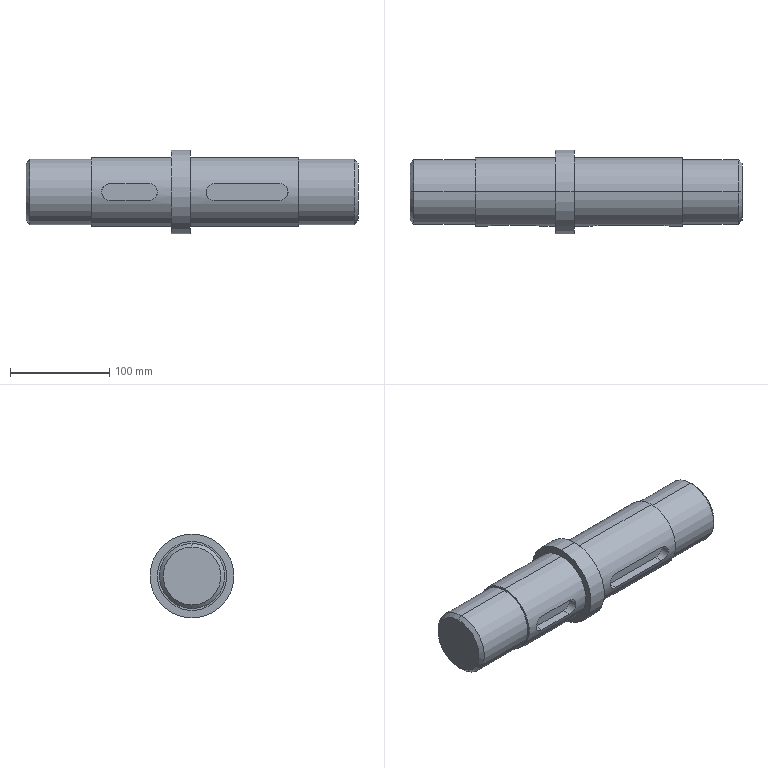Part | SolidWorks | features ICE 2, Chamfer 1, Revolution 1, Scale 1 | 1 solid | 30 faces | box 333.75 x 84.375 x 84.375 mm | volume 1222734 mm3 | cylinder 14 | plane 12 | cone 4 | commonest cylinder face diameters 16.875 x4 65.625 x4 69.375 x4 84.375 x2
STEP:
#1=CARTESIAN_POINT('',(-143.85,-0.2286,29.063));
#2=VERTEX_POINT('',#1);
#3=CARTESIAN_POINT('',(-143.85,-0.2286,-29.062));
#4=VERTEX_POINT('',#3);
#5=CARTESIAN_POINT('',(-143.85,-0.2286,0.000000086));
#6=DIRECTION('',(-1.,0.,0.));
#7=DIRECTION('',(0.,0.,-1.));
#8=AXIS2_PLACEMENT_3D('',#5,#6,#7);
#9=CIRCLE('',#8,29.062);
#10=EDGE_CURVE('',#2,#4,#9,.T.);
#11=ORIENTED_EDGE('',*,*,#10,.F.);
#12=CARTESIAN_POINT('',(-140.1,-0.2286,32.813));
#13=VERTEX_POINT('',#12);
#14=CARTESIAN_POINT('',(-143.85,-0.2286,29.063));
#15=DIRECTION('',(0.7071,0.,0.7071));
#16=VECTOR('',#15,1000.);
#17=LINE('',#14,#16);
#18=EDGE_CURVE('',#2,#13,#17,.T.);
#19=ORIENTED_EDGE('',*,*,#18,.T.);
#20=CARTESIAN_POINT('',(-140.1,-0.2286,-32.812));
#21=VERTEX_POINT('',#20);
#22=CARTESIAN_POINT('',(-140.1,-0.2286,0.000000086));
#23=DIRECTION('',(1.,0.,0.));
#24=DIRECTION('',(0.,0.,-1.));
#25=AXIS2_PLACEMENT_3D('',#22,#23,#24);
#26=CIRCLE('',#25,32.812);
#27=EDGE_CURVE('',#21,#13,#26,.T.);
#28=ORIENTED_EDGE('',*,*,#27,.F.);
#29=CARTESIAN_POINT('',(-143.85,-0.2286,-29.062));
#30=DIRECTION('',(0.7071,0.,-0.7071));
#31=VECTOR('',#30,1000.);
#32=LINE('',#29,#31);
#33=EDGE_CURVE('',#4,#21,#32,.T.);
#34=ORIENTED_EDGE('',*,*,#33,.F.);
#35=EDGE_LOOP('',(#11,#19,#28,#34));
#36=FACE_OUTER_BOUND('',#35,.T.);
#37=CARTESIAN_POINT('',(-143.85,-0.2286,0.000000086));
#38=DIRECTION('',(1.,0.,0.));
#39=DIRECTION('',(0.,0.,-1.));
#40=AXIS2_PLACEMENT_3D('',#37,#38,#39);
#41=CONICAL_SURFACE('',#40,29.062,0.7854);
#42=ADVANCED_FACE('',(#36),#41,.T.);
#43=CARTESIAN_POINT('',(189.9,-0.2286,-29.062));
#44=VERTEX_POINT('',#43);
#45=CARTESIAN_POINT('',(189.9,-0.2286,29.063));
#46=VERTEX_POINT('',#45);
#47=CARTESIAN_POINT('',(189.9,-0.2286,0.000000086));
#48=DIRECTION('',(1.,0.,0.));
#49=DIRECTION('',(0.,0.,1.));
#50=AXIS2_PLACEMENT_3D('',#47,#48,#49);
#51=CIRCLE('',#50,29.062);
#52=EDGE_CURVE('',#44,#46,#51,.T.);
#53=ORIENTED_EDGE('',*,*,#52,.F.);
#54=CARTESIAN_POINT('',(186.15,-0.2286,-32.812));
#55=VERTEX_POINT('',#54);
#56=CARTESIAN_POINT('',(186.15,-0.2286,-32.812));
#57=DIRECTION('',(-0.7071,0.,-0.7071));
#58=VECTOR('',#57,1000.);
#59=LINE('',#56,#58);
#60=EDGE_CURVE('',#44,#55,#59,.T.);
#61=ORIENTED_EDGE('',*,*,#60,.T.);
#62=CARTESIAN_POINT('',(186.15,-0.2286,32.813));
#63=VERTEX_POINT('',#62);
#64=CARTESIAN_POINT('',(186.15,-0.2286,0.000000086));
#65=DIRECTION('',(-1.,0.,0.));
#66=DIRECTION('',(0.,0.,1.));
#67=AXIS2_PLACEMENT_3D('',#64,#65,#66);
#68=CIRCLE('',#67,32.812);
#69=EDGE_CURVE('',#63,#55,#68,.T.);
#70=ORIENTED_EDGE('',*,*,#69,.F.);
#71=CARTESIAN_POINT('',(186.15,-0.2286,32.813));
#72=DIRECTION('',(-0.7071,0.,0.7071));
#73=VECTOR('',#72,1000.);
#74=LINE('',#71,#73);
#75=EDGE_CURVE('',#46,#63,#74,.T.);
#76=ORIENTED_EDGE('',*,*,#75,.F.);
#77=EDGE_LOOP('',(#53,#61,#70,#76));
#78=FACE_OUTER_BOUND('',#77,.T.);
#79=CARTESIAN_POINT('',(186.15,-0.2286,0.000000086));
#80=DIRECTION('',(-1.,0.,0.));
#81=DIRECTION('',(0.,0.,1.));
#82=AXIS2_PLACEMENT_3D('',#79,#80,#81);
#83=CONICAL_SURFACE('',#82,32.812,0.7854);
#84=ADVANCED_FACE('',(#78),#83,.T.);
#85=ORIENTED_EDGE('',*,*,#69,.T.);
#86=CARTESIAN_POINT('',(129.9,-0.2286,-32.812));
#87=VERTEX_POINT('',#86);
#88=CARTESIAN_POINT('',(-143.85,-0.2286,-32.812));
#89=DIRECTION('',(-1.,0.,0.));
#90=VECTOR('',#89,1000.);
#91=LINE('',#88,#90);
#92=EDGE_CURVE('',#55,#87,#91,.T.);
#93=ORIENTED_EDGE('',*,*,#92,.T.);
#94=CARTESIAN_POINT('',(129.9,-0.2286,32.813));
#95=VERTEX_POINT('',#94);
#96=CARTESIAN_POINT('',(129.9,-0.2286,0.000000086));
#97=DIRECTION('',(-1.,0.,0.));
#98=DIRECTION('',(0.,0.,1.));
#99=AXIS2_PLACEMENT_3D('',#96,#97,#98);
#100=CIRCLE('',#99,32.812);
#101=EDGE_CURVE('',#95,#87,#100,.T.);
#102=ORIENTED_EDGE('',*,*,#101,.F.);
#103=CARTESIAN_POINT('',(-143.85,-0.2286,32.813));
#104=DIRECTION('',(-1.,0.,0.));
#105=VECTOR('',#104,1000.);
#106=LINE('',#103,#105);
#107=EDGE_CURVE('',#63,#95,#106,.T.);
#108=ORIENTED_EDGE('',*,*,#107,.F.);
#109=EDGE_LOOP('',(#85,#93,#102,#108));
#110=FACE_OUTER_BOUND('',#109,.T.);
#111=CARTESIAN_POINT('',(-143.85,-0.2286,0.000000086));
#112=DIRECTION('',(-1.,0.,0.));
#113=DIRECTION('',(0.,0.,1.));
#114=AXIS2_PLACEMENT_3D('',#111,#112,#113);
#115=CYLINDRICAL_SURFACE('',#114,32.812);
#116=ADVANCED_FACE('',(#110),#115,.T.);
#117=CARTESIAN_POINT('',(129.9,-0.2286,34.688));
#118=VERTEX_POINT('',#117);
#119=CARTESIAN_POINT('',(129.9,-0.2286,-34.687));
#120=VERTEX_POINT('',#119);
#121=CARTESIAN_POINT('',(129.9,-0.2286,0.000000086));
#122=DIRECTION('',(-1.,0.,0.));
#123=DIRECTION('',(0.,0.,1.));
#124=AXIS2_PLACEMENT_3D('',#121,#122,#123);
#125=CIRCLE('',#124,34.688);
#126=EDGE_CURVE('',#118,#120,#125,.T.);
#127=ORIENTED_EDGE('',*,*,#126,.T.);
#128=CARTESIAN_POINT('',(21.15,-0.2286,-34.687));
#129=VERTEX_POINT('',#128);
#130=CARTESIAN_POINT('',(-143.85,-0.2286,-34.687));
#131=DIRECTION('',(-1.,0.,0.));
#132=VECTOR('',#131,1000.);
#133=LINE('',#130,#132);
#134=EDGE_CURVE('',#120,#129,#133,.T.);
#135=ORIENTED_EDGE('',*,*,#134,.T.);
#136=CARTESIAN_POINT('',(21.15,-0.2286,34.688));
#137=VERTEX_POINT('',#136);
#138=CARTESIAN_POINT('',(21.15,-0.2286,0.000000086));
#139=DIRECTION('',(-1.,0.,0.));
#140=DIRECTION('',(0.,0.,1.));
#141=AXIS2_PLACEMENT_3D('',#138,#139,#140);
#142=CIRCLE('',#141,34.688);
#143=EDGE_CURVE('',#137,#129,#142,.T.);
#144=ORIENTED_EDGE('',*,*,#143,.F.);
#145=CARTESIAN_POINT('',(-143.85,-0.2286,34.688));
#146=DIRECTION('',(-1.,0.,0.));
#147=VECTOR('',#146,1000.);
#148=LINE('',#145,#147);
#149=EDGE_CURVE('',#118,#137,#148,.T.);
#150=ORIENTED_EDGE('',*,*,#149,.F.);
#151=EDGE_LOOP('',(#127,#135,#144,#150));
#152=FACE_OUTER_BOUND('',#151,.T.);
#153=CARTESIAN_POINT('',(-143.85,-0.2286,0.000000086));
#154=DIRECTION('',(-1.,0.,0.));
#155=DIRECTION('',(0.,0.,1.));
#156=AXIS2_PLACEMENT_3D('',#153,#154,#155);
#157=CYLINDRICAL_SURFACE('',#156,34.688);
#158=ADVANCED_FACE('',(#152),#157,.T.);
#159=CARTESIAN_POINT('',(21.15,-0.2286,42.188));
#160=VERTEX_POINT('',#159);
#161=CARTESIAN_POINT('',(21.15,-0.2286,-42.187));
#162=VERTEX_POINT('',#161);
#163=CARTESIAN_POINT('',(21.15,-0.2286,0.000000086));
#164=DIRECTION('',(-1.,0.,0.));
#165=DIRECTION('',(0.,0.,1.));
#166=AXIS2_PLACEMENT_3D('',#163,#164,#165);
#167=CIRCLE('',#166,42.188);
#168=EDGE_CURVE('',#160,#162,#167,.T.);
#169=ORIENTED_EDGE('',*,*,#168,.T.);
#170=CARTESIAN_POINT('',(2.4,-0.2286,-42.187));
#171=VERTEX_POINT('',#170);
#172=CARTESIAN_POINT('',(-143.85,-0.2286,-42.187));
#173=DIRECTION('',(-1.,0.,0.));
#174=VECTOR('',#173,1000.);
#175=LINE('',#172,#174);
#176=EDGE_CURVE('',#162,#171,#175,.T.);
#177=ORIENTED_EDGE('',*,*,#176,.T.);
#178=CARTESIAN_POINT('',(2.4,-0.2286,42.188));
#179=VERTEX_POINT('',#178);
#180=CARTESIAN_POINT('',(2.4,-0.2286,0.000000086));
#181=DIRECTION('',(-1.,0.,0.));
#182=DIRECTION('',(0.,0.,1.));
#183=AXIS2_PLACEMENT_3D('',#180,#181,#182);
#184=CIRCLE('',#183,42.188);
#185=EDGE_CURVE('',#179,#171,#184,.T.);
#186=ORIENTED_EDGE('',*,*,#185,.F.);
#187=CARTESIAN_POINT('',(-143.85,-0.2286,42.188));
#188=DIRECTION('',(-1.,0.,0.));
#189=VECTOR('',#188,1000.);
#190=LINE('',#187,#189);
#191=EDGE_CURVE('',#160,#179,#190,.T.);
#192=ORIENTED_EDGE('',*,*,#191,.F.);
#193=EDGE_LOOP('',(#169,#177,#186,#192));
#194=FACE_OUTER_BOUND('',#193,.T.);
#195=CARTESIAN_POINT('',(-143.85,-0.2286,0.000000086));
#196=DIRECTION('',(-1.,0.,0.));
#197=DIRECTION('',(0.,0.,1.));
#198=AXIS2_PLACEMENT_3D('',#195,#196,#197);
#199=CYLINDRICAL_SURFACE('',#198,42.188);
#200=ADVANCED_FACE('',(#194),#199,.T.);
#201=CARTESIAN_POINT('',(2.4,-0.2286,34.688));
#202=VERTEX_POINT('',#201);
#203=CARTESIAN_POINT('',(2.4,-0.2286,-34.687));
#204=VERTEX_POINT('',#203);
#205=CARTESIAN_POINT('',(2.4,-0.2286,0.000000086));
#206=DIRECTION('',(-1.,0.,0.));
#207=DIRECTION('',(0.,0.,1.));
#208=AXIS2_PLACEMENT_3D('',#205,#206,#207);
#209=CIRCLE('',#208,34.688);
#210=EDGE_CURVE('',#202,#204,#209,.T.);
#211=ORIENTED_EDGE('',*,*,#210,.T.);
#212=CARTESIAN_POINT('',(-78.225,-0.2286,-34.687));
#213=VERTEX_POINT('',#212);
#214=CARTESIAN_POINT('',(-143.85,-0.2286,-34.687));
#215=DIRECTION('',(-1.,0.,0.));
#216=VECTOR('',#215,1000.);
#217=LINE('',#214,#216);
#218=EDGE_CURVE('',#204,#213,#217,.T.);
#219=ORIENTED_EDGE('',*,*,#218,.T.);
#220=CARTESIAN_POINT('',(-78.225,-0.2286,34.688));
#221=VERTEX_POINT('',#220);
#222=CARTESIAN_POINT('',(-78.225,-0.2286,0.000000086));
#223=DIRECTION('',(-1.,0.,0.));
#224=DIRECTION('',(0.,0.,1.));
#225=AXIS2_PLACEMENT_3D('',#222,#223,#224);
#226=CIRCLE('',#225,34.688);
#227=EDGE_CURVE('',#221,#213,#226,.T.);
#228=ORIENTED_EDGE('',*,*,#227,.F.);
#229=CARTESIAN_POINT('',(-143.85,-0.2286,34.688));
#230=DIRECTION('',(-1.,0.,0.));
#231=VECTOR('',#230,1000.);
#232=LINE('',#229,#231);
#233=EDGE_CURVE('',#202,#221,#232,.T.);
#234=ORIENTED_EDGE('',*,*,#233,.F.);
#235=EDGE_LOOP('',(#211,#219,#228,#234));
#236=FACE_OUTER_BOUND('',#235,.T.);
#237=CARTESIAN_POINT('',(-143.85,-0.2286,0.000000086));
#238=DIRECTION('',(-1.,0.,0.));
#239=DIRECTION('',(0.,0.,1.));
#240=AXIS2_PLACEMENT_3D('',#237,#238,#239);
#241=CYLINDRICAL_SURFACE('',#240,34.688);
#242=ADVANCED_FACE('',(#236),#241,.T.);
#243=CARTESIAN_POINT('',(-78.225,-0.2286,32.813));
#244=VERTEX_POINT('',#243);
#245=CARTESIAN_POINT('',(-78.225,-0.2286,-32.812));
#246=VERTEX_POINT('',#245);
#247=CARTESIAN_POINT('',(-78.225,-0.2286,0.000000086));
#248=DIRECTION('',(-1.,0.,0.));
#249=DIRECTION('',(0.,0.,1.));
#250=AXIS2_PLACEMENT_3D('',#247,#248,#249);
#251=CIRCLE('',#250,32.812);
#252=EDGE_CURVE('',#244,#246,#251,.T.);
#253=ORIENTED_EDGE('',*,*,#252,.T.);
#254=CARTESIAN_POINT('',(-143.85,-0.2286,-32.812));
#255=DIRECTION('',(-1.,0.,0.));
#256=VECTOR('',#255,1000.);
#257=LINE('',#254,#256);
#258=EDGE_CURVE('',#246,#21,#257,.T.);
#259=ORIENTED_EDGE('',*,*,#258,.T.);
#260=ORIENTED_EDGE('',*,*,#27,.T.);
#261=CARTESIAN_POINT('',(-143.85,-0.2286,32.813));
#262=DIRECTION('',(-1.,0.,0.));
#263=VECTOR('',#262,1000.);
#264=LINE('',#261,#263);
#265=EDGE_CURVE('',#244,#13,#264,.T.);
#266=ORIENTED_EDGE('',*,*,#265,.F.);
#267=EDGE_LOOP('',(#253,#259,#260,#266));
#268=FACE_OUTER_BOUND('',#267,.T.);
#269=CARTESIAN_POINT('',(-143.85,-0.2286,0.000000086));
#270=DIRECTION('',(-1.,0.,0.));
#271=DIRECTION('',(0.,0.,1.));
#272=AXIS2_PLACEMENT_3D('',#269,#270,#271);
#273=CYLINDRICAL_SURFACE('',#272,32.812);
#274=ADVANCED_FACE('',(#268),#273,.T.);
#275=CARTESIAN_POINT('',(45.525,-25.541,-8.437));
#276=VERTEX_POINT('',#275);
#277=CARTESIAN_POINT('',(45.525,-25.541,8.438));
#278=VERTEX_POINT('',#277);
#279=CARTESIAN_POINT('',(45.525,-25.541,0.000000086));
#280=DIRECTION('',(0.,1.,0.));
#281=DIRECTION('',(0.,0.,1.));
#282=AXIS2_PLACEMENT_3D('',#279,#280,#281);
#283=CIRCLE('',#282,8.438);
#284=EDGE_CURVE('',#276,#278,#283,.T.);
#285=ORIENTED_EDGE('',*,*,#284,.T.);
#286=CARTESIAN_POINT('',(45.525,-33.874,8.438));
#287=VERTEX_POINT('',#286);
#288=CARTESIAN_POINT('',(45.525,-165.229,8.438));
#289=DIRECTION('',(0.,1.,0.));
#290=VECTOR('',#289,1000.);
#291=LINE('',#288,#290);
#292=EDGE_CURVE('',#287,#278,#291,.T.);
#293=ORIENTED_EDGE('',*,*,#292,.F.);
#294=CARTESIAN_POINT('',(45.525,-33.874,-8.437));
#295=VERTEX_POINT('',#294);
#296=CARTESIAN_POINT('',(45.525,-33.874,-8.437));
#297=CARTESIAN_POINT('',(44.973,-33.874,-8.437));
#298=CARTESIAN_POINT('',(44.423,-33.888,-8.384));
#299=CARTESIAN_POINT('',(43.327,-33.942,-8.165));
#300=CARTESIAN_POINT('',(42.799,-33.981,-8.004));
#301=CARTESIAN_POINT('',(42.037,-34.054,-7.688));
#302=CARTESIAN_POINT('',(41.788,-34.08,-7.57));
#303=CARTESIAN_POINT('',(41.3,-34.138,-7.309));
#304=CARTESIAN_POINT('',(41.061,-34.168,-7.165));
#305=CARTESIAN_POINT('',(40.374,-34.263,-6.706));
#306=CARTESIAN_POINT('',(39.951,-34.331,-6.358));
#307=CARTESIAN_POINT('',(39.367,-34.433,-5.775));
#308=CARTESIAN_POINT('',(39.18,-34.467,-5.569));
#309=CARTESIAN_POINT('',(38.829,-34.534,-5.142));
#310=CARTESIAN_POINT('',(38.665,-34.566,-4.921));
#311=CARTESIAN_POINT('',(38.208,-34.659,-4.237));
#312=CARTESIAN_POINT('',(37.948,-34.716,-3.753));
#313=CARTESIAN_POINT('',(37.628,-34.789,-2.984));
#314=CARTESIAN_POINT('',(37.534,-34.81,-2.721));
#315=CARTESIAN_POINT('',(37.373,-34.848,-2.193));
#316=CARTESIAN_POINT('',(37.238,-34.88,-1.659));
#317=CARTESIAN_POINT('',(37.157,-34.899,-1.113));
#318=CARTESIAN_POINT('',(37.102,-34.913,-0.5614));
#319=CARTESIAN_POINT('',(37.088,-34.916,-0.2811));
#320=CARTESIAN_POINT('',(37.087,-34.916,0.5538));
#321=CARTESIAN_POINT('',(37.142,-34.903,1.103));
#322=CARTESIAN_POINT('',(37.357,-34.851,2.186));
#323=CARTESIAN_POINT('',(37.521,-34.813,2.725));
#324=CARTESIAN_POINT('',(37.943,-34.717,3.743));
#325=CARTESIAN_POINT('',(38.202,-34.661,4.227));
#326=CARTESIAN_POINT('',(38.663,-34.567,4.917));
#327=CARTESIAN_POINT('',(38.829,-34.534,5.141));
#328=CARTESIAN_POINT('',(39.178,-34.467,5.566));
#329=CARTESIAN_POINT('',(39.362,-34.434,5.769));
#330=CARTESIAN_POINT('',(39.749,-34.366,6.157));
#331=CARTESIAN_POINT('',(39.952,-34.332,6.341));
#332=CARTESIAN_POINT('',(40.377,-34.265,6.691));
#333=CARTESIAN_POINT('',(40.6,-34.232,6.857));
#334=CARTESIAN_POINT('',(41.29,-34.137,7.319));
#335=CARTESIAN_POINT('',(41.774,-34.079,7.578));
#336=CARTESIAN_POINT('',(42.535,-34.006,7.895));
#337=CARTESIAN_POINT('',(42.795,-33.984,7.989));
#338=CARTESIAN_POINT('',(43.327,-33.945,8.151));
#339=CARTESIAN_POINT('',(43.598,-33.928,8.219));
#340=CARTESIAN_POINT('',(44.414,-33.888,8.382));
#341=CARTESIAN_POINT('',(44.965,-33.874,8.438));
#342=CARTESIAN_POINT('',(45.525,-33.874,8.438));
#343=B_SPLINE_CURVE_WITH_KNOTS('',3,(#296,#297,#298,#299,#300,#301,#302,#303,#304,#305,#306,#307,#308,#309,#310,#311,#312,#313,#314,#315,#316,#317,#318,#319,#320,#321,#322,#323,#324,#325,#326,#327,#328,#329,#330,#331,#332,#333,#334,#335,#336,#337,#338,#339,#340,#341,#342),.UNSPECIFIED.,.F.,.F.,(4,2,2,2,2,2,2,2,2,2,1,2,2,2,2,2,2,2,2,2,2,2,2,4),(0.02648,0.02813,0.02979,0.03062,0.03144,0.0331,0.03392,0.03475,0.03641,0.03723,0.03806,0.03889,0.03971,0.04137,0.04302,0.04468,0.04551,0.04633,0.04716,0.04799,0.04964,0.05047,0.0513,0.05295),.UNSPECIFIED.);
#344=EDGE_CURVE('',#295,#287,#343,.T.);
#345=ORIENTED_EDGE('',*,*,#344,.F.);
#346=CARTESIAN_POINT('',(45.525,-165.229,-8.437));
#347=DIRECTION('',(0.,1.,0.));
#348=VECTOR('',#347,1000.);
#349=LINE('',#346,#348);
#350=EDGE_CURVE('',#295,#276,#349,.T.);
#351=ORIENTED_EDGE('',*,*,#350,.T.);
#352=EDGE_LOOP('',(#285,#293,#345,#351));
#353=FACE_OUTER_BOUND('',#352,.T.);
#354=CARTESIAN_POINT('',(45.525,-165.229,0.000000086));
#355=DIRECTION('',(0.,1.,0.));
#356=DIRECTION('',(0.,0.,1.));
#357=AXIS2_PLACEMENT_3D('',#354,#355,#356);
#358=CYLINDRICAL_SURFACE('',#357,8.438);
#359=ADVANCED_FACE('',(#353),#358,.F.);
#360=CARTESIAN_POINT('',(111.15,-25.541,-8.437));
#361=VERTEX_POINT('',#360);
#362=CARTESIAN_POINT('',(45.525,-25.541,-8.437));
#363=DIRECTION('',(-1.,0.,0.));
#364=VECTOR('',#363,1000.);
#365=LINE('',#362,#364);
#366=EDGE_CURVE('',#361,#276,#365,.T.);
#367=ORIENTED_EDGE('',*,*,#366,.T.);
#368=ORIENTED_EDGE('',*,*,#350,.F.);
#369=CARTESIAN_POINT('',(111.15,-33.874,-8.437));
#370=VERTEX_POINT('',#369);
#371=CARTESIAN_POINT('',(-143.85,-33.874,-8.437));
#372=DIRECTION('',(-1.,0.,0.));
#373=VECTOR('',#372,1000.);
#374=LINE('',#371,#373);
#375=EDGE_CURVE('',#370,#295,#374,.T.);
#376=ORIENTED_EDGE('',*,*,#375,.F.);
#377=CARTESIAN_POINT('',(111.15,-165.229,-8.437));
#378=DIRECTION('',(0.,1.,0.));
#379=VECTOR('',#378,1000.);
#380=LINE('',#377,#379);
#381=EDGE_CURVE('',#370,#361,#380,.T.);
#382=ORIENTED_EDGE('',*,*,#381,.T.);
#383=EDGE_LOOP('',(#367,#368,#376,#382));
#384=FACE_OUTER_BOUND('',#383,.T.);
#385=CARTESIAN_POINT('',(45.525,-165.229,-8.437));
#386=DIRECTION('',(0.,0.,-1.));
#387=DIRECTION('',(-1.,0.,0.));
#388=AXIS2_PLACEMENT_3D('',#385,#386,#387);
#389=PLANE('',#388);
#390=ADVANCED_FACE('',(#384),#389,.F.);
#391=CARTESIAN_POINT('',(111.15,-25.541,8.438));
#392=VERTEX_POINT('',#391);
#393=CARTESIAN_POINT('',(111.15,-25.541,0.000000086));
#394=DIRECTION('',(0.,1.,0.));
#395=DIRECTION('',(0.,0.,1.));
#396=AXIS2_PLACEMENT_3D('',#393,#394,#395);
#397=CIRCLE('',#396,8.438);
#398=EDGE_CURVE('',#392,#361,#397,.T.);
#399=ORIENTED_EDGE('',*,*,#398,.T.);
#400=ORIENTED_EDGE('',*,*,#381,.F.);
#401=CARTESIAN_POINT('',(111.15,-33.874,8.438));
#402=VERTEX_POINT('',#401);
#403=CARTESIAN_POINT('',(111.15,-33.874,8.438));
#404=CARTESIAN_POINT('',(111.71,-33.874,8.438));
#405=CARTESIAN_POINT('',(112.26,-33.888,8.382));
#406=CARTESIAN_POINT('',(113.071,-33.928,8.221));
#407=CARTESIAN_POINT('',(113.339,-33.944,8.153));
#408=CARTESIAN_POINT('',(113.87,-33.983,7.992));
#409=CARTESIAN_POINT('',(114.133,-34.005,7.897));
#410=CARTESIAN_POINT('',(114.899,-34.079,7.579));
#411=CARTESIAN_POINT('',(115.383,-34.136,7.32));
#412=CARTESIAN_POINT('',(116.069,-34.231,6.861));
#413=CARTESIAN_POINT('',(116.293,-34.264,6.695));
#414=CARTESIAN_POINT('',(116.72,-34.332,6.344));
#415=CARTESIAN_POINT('',(116.924,-34.366,6.159));
#416=CARTESIAN_POINT('',(117.505,-34.467,5.577));
#417=CARTESIAN_POINT('',(117.854,-34.534,5.154));
#418=CARTESIAN_POINT('',(118.316,-34.629,4.462));
#419=CARTESIAN_POINT('',(118.459,-34.659,4.224));
#420=CARTESIAN_POINT('',(118.719,-34.715,3.739));
#421=CARTESIAN_POINT('',(118.837,-34.741,3.49));
#422=CARTESIAN_POINT('',(119.047,-34.789,2.983));
#423=CARTESIAN_POINT('',(119.14,-34.81,2.724));
#424=CARTESIAN_POINT('',(119.302,-34.848,2.195));
#425=CARTESIAN_POINT('',(119.37,-34.864,1.923));
#426=CARTESIAN_POINT('',(119.533,-34.903,1.105));
#427=CARTESIAN_POINT('',(119.587,-34.916,0.5561));
#428=CARTESIAN_POINT('',(119.588,-34.916,-0.5493));
#429=CARTESIAN_POINT('',(119.532,-34.903,-1.111));
#430=CARTESIAN_POINT('',(119.316,-34.851,-2.195));
#431=CARTESIAN_POINT('',(119.156,-34.813,-2.722));
#432=CARTESIAN_POINT('',(118.837,-34.741,-3.49));
#433=CARTESIAN_POINT('',(118.717,-34.715,-3.743));
#434=CARTESIAN_POINT('',(118.456,-34.658,-4.229));
#435=CARTESIAN_POINT('',(118.315,-34.628,-4.465));
#436=CARTESIAN_POINT('',(118.01,-34.566,-4.92));
#437=CARTESIAN_POINT('',(117.846,-34.534,-5.141));
#438=CARTESIAN_POINT('',(117.497,-34.467,-5.566));
#439=CARTESIAN_POINT('',(117.31,-34.433,-5.772));
#440=CARTESIAN_POINT('',(116.723,-34.331,-6.359));
#441=CARTESIAN_POINT('',(116.3,-34.263,-6.706));
#442=CARTESIAN_POINT('',(115.615,-34.169,-7.164));
#443=CARTESIAN_POINT('',(115.379,-34.138,-7.306));
#444=CARTESIAN_POINT('',(114.89,-34.081,-7.568));
#445=CARTESIAN_POINT('',(114.638,-34.054,-7.688));
#446=CARTESIAN_POINT('',(113.874,-33.981,-8.005));
#447=CARTESIAN_POINT('',(113.348,-33.942,-8.165));
#448=CARTESIAN_POINT('',(112.534,-33.902,-8.328));
#449=CARTESIAN_POINT('',(112.256,-33.891,-8.369));
#450=CARTESIAN_POINT('',(111.702,-33.878,-8.424));
#451=CARTESIAN_POINT('',(111.426,-33.874,-8.437));
#452=CARTESIAN_POINT('',(111.15,-33.874,-8.437));
#453=B_SPLINE_CURVE_WITH_KNOTS('',3,(#403,#404,#405,#406,#407,#408,#409,#410,#411,#412,#413,#414,#415,#416,#417,#418,#419,#420,#421,#422,#423,#424,#425,#426,#427,#428,#429,#430,#431,#432,#433,#434,#435,#436,#437,#438,#439,#440,#441,#442,#443,#444,#445,#446,#447,#448,#449,#450,#451,#452),.UNSPECIFIED.,.F.,.F.,(4,2,2,2,2,2,2,2,2,2,2,2,2,2,2,2,2,2,2,2,2,2,2,2,4),(0.,0.001655,0.002482,0.00331,0.004965,0.005792,0.00662,0.008275,0.009102,0.00993,0.01076,0.01158,0.01324,0.01489,0.01655,0.01738,0.0182,0.01903,0.01986,0.02151,0.02234,0.02317,0.02482,0.02565,0.02648),.UNSPECIFIED.);
#454=EDGE_CURVE('',#402,#370,#453,.T.);
#455=ORIENTED_EDGE('',*,*,#454,.F.);
#456=CARTESIAN_POINT('',(111.15,-165.229,8.438));
#457=DIRECTION('',(0.,1.,0.));
#458=VECTOR('',#457,1000.);
#459=LINE('',#456,#458);
#460=EDGE_CURVE('',#402,#392,#459,.T.);
#461=ORIENTED_EDGE('',*,*,#460,.T.);
#462=EDGE_LOOP('',(#399,#400,#455,#461));
#463=FACE_OUTER_BOUND('',#462,.T.);
#464=CARTESIAN_POINT('',(111.15,-165.229,0.000000086));
#465=DIRECTION('',(0.,1.,0.));
#466=DIRECTION('',(0.,0.,1.));
#467=AXIS2_PLACEMENT_3D('',#464,#465,#466);
#468=CYLINDRICAL_SURFACE('',#467,8.438);
#469=ADVANCED_FACE('',(#463),#468,.F.);
#470=CARTESIAN_POINT('',(45.525,-25.541,8.438));
#471=DIRECTION('',(1.,0.,0.));
#472=VECTOR('',#471,1000.);
#473=LINE('',#470,#472);
#474=EDGE_CURVE('',#278,#392,#473,.T.);
#475=ORIENTED_EDGE('',*,*,#474,.T.);
#476=ORIENTED_EDGE('',*,*,#460,.F.);
#477=CARTESIAN_POINT('',(-143.85,-33.874,8.438));
#478=DIRECTION('',(1.,0.,0.));
#479=VECTOR('',#478,1000.);
#480=LINE('',#477,#479);
#481=EDGE_CURVE('',#287,#402,#480,.T.);
#482=ORIENTED_EDGE('',*,*,#481,.F.);
#483=ORIENTED_EDGE('',*,*,#292,.T.);
#484=EDGE_LOOP('',(#475,#476,#482,#483));
#485=FACE_OUTER_BOUND('',#484,.T.);
#486=CARTESIAN_POINT('',(45.525,-165.229,8.438));
#487=DIRECTION('',(0.,0.,1.));
#488=DIRECTION('',(1.,0.,0.));
#489=AXIS2_PLACEMENT_3D('',#486,#487,#488);
#490=PLANE('',#489);
#491=ADVANCED_FACE('',(#485),#490,.F.);
#492=CARTESIAN_POINT('',(-59.475,-25.541,-8.437));
#493=VERTEX_POINT('',#492);
#494=CARTESIAN_POINT('',(-59.475,-25.541,8.438));
#495=VERTEX_POINT('',#494);
#496=CARTESIAN_POINT('',(-59.475,-25.541,0.000000086));
#497=DIRECTION('',(0.,1.,0.));
#498=DIRECTION('',(0.,0.,1.));
#499=AXIS2_PLACEMENT_3D('',#496,#497,#498);
#500=CIRCLE('',#499,8.437);
#501=EDGE_CURVE('',#493,#495,#500,.T.);
#502=ORIENTED_EDGE('',*,*,#501,.T.);
#503=CARTESIAN_POINT('',(-59.475,-33.874,8.438));
#504=VERTEX_POINT('',#503);
#505=CARTESIAN_POINT('',(-59.475,-165.229,8.438));
#506=DIRECTION('',(0.,1.,0.));
#507=VECTOR('',#506,1000.);
#508=LINE('',#505,#507);
#509=EDGE_CURVE('',#504,#495,#508,.T.);
#510=ORIENTED_EDGE('',*,*,#509,.F.);
#511=CARTESIAN_POINT('',(-59.475,-33.874,-8.437));
#512=VERTEX_POINT('',#511);
#513=CARTESIAN_POINT('',(-59.475,-33.874,-8.437));
#514=CARTESIAN_POINT('',(-60.027,-33.874,-8.437));
#515=CARTESIAN_POINT('',(-60.577,-33.888,-8.384));
#516=CARTESIAN_POINT('',(-61.673,-33.942,-8.165));
#517=CARTESIAN_POINT('',(-62.201,-33.981,-8.004));
#518=CARTESIAN_POINT('',(-62.963,-34.054,-7.688));
#519=CARTESIAN_POINT('',(-63.212,-34.08,-7.57));
#520=CARTESIAN_POINT('',(-63.7,-34.138,-7.309));
#521=CARTESIAN_POINT('',(-63.939,-34.168,-7.165));
#522=CARTESIAN_POINT('',(-64.626,-34.263,-6.706));
#523=CARTESIAN_POINT('',(-65.049,-34.331,-6.358));
#524=CARTESIAN_POINT('',(-65.633,-34.433,-5.775));
#525=CARTESIAN_POINT('',(-65.82,-34.467,-5.569));
#526=CARTESIAN_POINT('',(-66.171,-34.534,-5.142));
#527=CARTESIAN_POINT('',(-66.335,-34.566,-4.921));
#528=CARTESIAN_POINT('',(-66.792,-34.659,-4.237));
#529=CARTESIAN_POINT('',(-67.052,-34.716,-3.753));
#530=CARTESIAN_POINT('',(-67.372,-34.789,-2.984));
#531=CARTESIAN_POINT('',(-67.466,-34.81,-2.721));
#532=CARTESIAN_POINT('',(-67.627,-34.848,-2.193));
#533=CARTESIAN_POINT('',(-67.762,-34.88,-1.659));
#534=CARTESIAN_POINT('',(-67.843,-34.899,-1.113));
#535=CARTESIAN_POINT('',(-67.898,-34.913,-0.5614));
#536=CARTESIAN_POINT('',(-67.912,-34.916,-0.2811));
#537=CARTESIAN_POINT('',(-67.913,-34.916,0.5538));
#538=CARTESIAN_POINT('',(-67.858,-34.903,1.103));
#539=CARTESIAN_POINT('',(-67.643,-34.851,2.186));
#540=CARTESIAN_POINT('',(-67.479,-34.813,2.725));
#541=CARTESIAN_POINT('',(-67.057,-34.717,3.743));
#542=CARTESIAN_POINT('',(-66.798,-34.661,4.227));
#543=CARTESIAN_POINT('',(-66.337,-34.567,4.917));
#544=CARTESIAN_POINT('',(-66.171,-34.534,5.141));
#545=CARTESIAN_POINT('',(-65.822,-34.467,5.566));
#546=CARTESIAN_POINT('',(-65.638,-34.434,5.769));
#547=CARTESIAN_POINT('',(-65.251,-34.366,6.157));
#548=CARTESIAN_POINT('',(-65.048,-34.332,6.341));
#549=CARTESIAN_POINT('',(-64.623,-34.265,6.691));
#550=CARTESIAN_POINT('',(-64.4,-34.232,6.857));
#551=CARTESIAN_POINT('',(-63.71,-34.137,7.319));
#552=CARTESIAN_POINT('',(-63.226,-34.079,7.578));
#553=CARTESIAN_POINT('',(-62.465,-34.006,7.895));
#554=CARTESIAN_POINT('',(-62.205,-33.984,7.989));
#555=CARTESIAN_POINT('',(-61.673,-33.945,8.151));
#556=CARTESIAN_POINT('',(-61.402,-33.928,8.219));
#557=CARTESIAN_POINT('',(-60.586,-33.888,8.382));
#558=CARTESIAN_POINT('',(-60.035,-33.874,8.438));
#559=CARTESIAN_POINT('',(-59.475,-33.874,8.438));
#560=B_SPLINE_CURVE_WITH_KNOTS('',3,(#513,#514,#515,#516,#517,#518,#519,#520,#521,#522,#523,#524,#525,#526,#527,#528,#529,#530,#531,#532,#533,#534,#535,#536,#537,#538,#539,#540,#541,#542,#543,#544,#545,#546,#547,#548,#549,#550,#551,#552,#553,#554,#555,#556,#557,#558,#559),.UNSPECIFIED.,.F.,.F.,(4,2,2,2,2,2,2,2,2,2,1,2,2,2,2,2,2,2,2,2,2,2,2,4),(0.02648,0.02813,0.02979,0.03062,0.03144,0.0331,0.03392,0.03475,0.03641,0.03723,0.03806,0.03889,0.03971,0.04137,0.04302,0.04468,0.04551,0.04633,0.04716,0.04799,0.04964,0.05047,0.0513,0.05295),.UNSPECIFIED.);
#561=EDGE_CURVE('',#512,#504,#560,.T.);
#562=ORIENTED_EDGE('',*,*,#561,.F.);
#563=CARTESIAN_POINT('',(-59.475,-165.229,-8.437));
#564=DIRECTION('',(0.,1.,0.));
#565=VECTOR('',#564,1000.);
#566=LINE('',#563,#565);
#567=EDGE_CURVE('',#512,#493,#566,.T.);
#568=ORIENTED_EDGE('',*,*,#567,.T.);
#569=EDGE_LOOP('',(#502,#510,#562,#568));
#570=FACE_OUTER_BOUND('',#569,.T.);
#571=CARTESIAN_POINT('',(-59.475,-165.229,0.000000086));
#572=DIRECTION('',(0.,1.,0.));
#573=DIRECTION('',(0.,0.,1.));
#574=AXIS2_PLACEMENT_3D('',#571,#572,#573);
#575=CYLINDRICAL_SURFACE('',#574,8.437);
#576=ADVANCED_FACE('',(#570),#575,.F.);
#577=CARTESIAN_POINT('',(-20.1,-25.541,-8.437));
#578=VERTEX_POINT('',#577);
#579=CARTESIAN_POINT('',(-59.475,-25.541,-8.437));
#580=DIRECTION('',(-1.,0.,0.));
#581=VECTOR('',#580,1000.);
#582=LINE('',#579,#581);
#583=EDGE_CURVE('',#578,#493,#582,.T.);
#584=ORIENTED_EDGE('',*,*,#583,.T.);
#585=ORIENTED_EDGE('',*,*,#567,.F.);
#586=CARTESIAN_POINT('',(-20.1,-33.874,-8.437));
#587=VERTEX_POINT('',#586);
#588=CARTESIAN_POINT('',(-143.85,-33.874,-8.437));
#589=DIRECTION('',(-1.,0.,0.));
#590=VECTOR('',#589,1000.);
#591=LINE('',#588,#590);
#592=EDGE_CURVE('',#587,#512,#591,.T.);
#593=ORIENTED_EDGE('',*,*,#592,.F.);
#594=CARTESIAN_POINT('',(-20.1,-165.229,-8.437));
#595=DIRECTION('',(0.,1.,0.));
#596=VECTOR('',#595,1000.);
#597=LINE('',#594,#596);
#598=EDGE_CURVE('',#587,#578,#597,.T.);
#599=ORIENTED_EDGE('',*,*,#598,.T.);
#600=EDGE_LOOP('',(#584,#585,#593,#599));
#601=FACE_OUTER_BOUND('',#600,.T.);
#602=CARTESIAN_POINT('',(-59.475,-165.229,-8.437));
#603=DIRECTION('',(0.,0.,-1.));
#604=DIRECTION('',(-1.,0.,0.));
#605=AXIS2_PLACEMENT_3D('',#602,#603,#604);
#606=PLANE('',#605);
#607=ADVANCED_FACE('',(#601),#606,.F.);
#608=CARTESIAN_POINT('',(-20.1,-25.541,8.438));
#609=VERTEX_POINT('',#608);
#610=CARTESIAN_POINT('',(-20.1,-25.541,0.000000086));
#611=DIRECTION('',(0.,1.,0.));
#612=DIRECTION('',(0.,0.,1.));
#613=AXIS2_PLACEMENT_3D('',#610,#611,#612);
#614=CIRCLE('',#613,8.438);
#615=EDGE_CURVE('',#609,#578,#614,.T.);
#616=ORIENTED_EDGE('',*,*,#615,.T.);
#617=ORIENTED_EDGE('',*,*,#598,.F.);
#618=CARTESIAN_POINT('',(-20.1,-33.874,8.438));
#619=VERTEX_POINT('',#618);
#620=CARTESIAN_POINT('',(-20.1,-33.874,8.438));
#621=CARTESIAN_POINT('',(-19.54,-33.874,8.438));
#622=CARTESIAN_POINT('',(-18.99,-33.888,8.382));
#623=CARTESIAN_POINT('',(-18.179,-33.928,8.221));
#624=CARTESIAN_POINT('',(-17.911,-33.944,8.153));
#625=CARTESIAN_POINT('',(-17.38,-33.983,7.992));
#626=CARTESIAN_POINT('',(-17.117,-34.005,7.897));
#627=CARTESIAN_POINT('',(-16.351,-34.079,7.579));
#628=CARTESIAN_POINT('',(-15.867,-34.136,7.32));
#629=CARTESIAN_POINT('',(-15.181,-34.231,6.861));
#630=CARTESIAN_POINT('',(-14.957,-34.264,6.695));
#631=CARTESIAN_POINT('',(-14.53,-34.332,6.344));
#632=CARTESIAN_POINT('',(-14.326,-34.366,6.159));
#633=CARTESIAN_POINT('',(-13.745,-34.467,5.577));
#634=CARTESIAN_POINT('',(-13.396,-34.534,5.154));
#635=CARTESIAN_POINT('',(-12.934,-34.629,4.462));
#636=CARTESIAN_POINT('',(-12.791,-34.659,4.224));
#637=CARTESIAN_POINT('',(-12.531,-34.715,3.739));
#638=CARTESIAN_POINT('',(-12.413,-34.741,3.49));
#639=CARTESIAN_POINT('',(-12.203,-34.789,2.983));
#640=CARTESIAN_POINT('',(-12.11,-34.81,2.724));
#641=CARTESIAN_POINT('',(-11.948,-34.848,2.195));
#642=CARTESIAN_POINT('',(-11.88,-34.864,1.923));
#643=CARTESIAN_POINT('',(-11.717,-34.903,1.105));
#644=CARTESIAN_POINT('',(-11.663,-34.916,0.5561));
#645=CARTESIAN_POINT('',(-11.662,-34.916,-0.5493));
#646=CARTESIAN_POINT('',(-11.718,-34.903,-1.111));
#647=CARTESIAN_POINT('',(-11.934,-34.851,-2.195));
#648=CARTESIAN_POINT('',(-12.094,-34.813,-2.722));
#649=CARTESIAN_POINT('',(-12.413,-34.741,-3.49));
#650=CARTESIAN_POINT('',(-12.533,-34.715,-3.743));
#651=CARTESIAN_POINT('',(-12.794,-34.658,-4.229));
#652=CARTESIAN_POINT('',(-12.935,-34.628,-4.465));
#653=CARTESIAN_POINT('',(-13.24,-34.566,-4.92));
#654=CARTESIAN_POINT('',(-13.404,-34.534,-5.141));
#655=CARTESIAN_POINT('',(-13.753,-34.467,-5.566));
#656=CARTESIAN_POINT('',(-13.94,-34.433,-5.772));
#657=CARTESIAN_POINT('',(-14.527,-34.331,-6.359));
#658=CARTESIAN_POINT('',(-14.95,-34.263,-6.706));
#659=CARTESIAN_POINT('',(-15.635,-34.169,-7.164));
#660=CARTESIAN_POINT('',(-15.871,-34.138,-7.306));
#661=CARTESIAN_POINT('',(-16.36,-34.081,-7.568));
#662=CARTESIAN_POINT('',(-16.612,-34.054,-7.688));
#663=CARTESIAN_POINT('',(-17.376,-33.981,-8.005));
#664=CARTESIAN_POINT('',(-17.902,-33.942,-8.165));
#665=CARTESIAN_POINT('',(-18.716,-33.902,-8.328));
#666=CARTESIAN_POINT('',(-18.994,-33.891,-8.369));
#667=CARTESIAN_POINT('',(-19.548,-33.878,-8.424));
#668=CARTESIAN_POINT('',(-19.824,-33.874,-8.437));
#669=CARTESIAN_POINT('',(-20.1,-33.874,-8.437));
#670=B_SPLINE_CURVE_WITH_KNOTS('',3,(#620,#621,#622,#623,#624,#625,#626,#627,#628,#629,#630,#631,#632,#633,#634,#635,#636,#637,#638,#639,#640,#641,#642,#643,#644,#645,#646,#647,#648,#649,#650,#651,#652,#653,#654,#655,#656,#657,#658,#659,#660,#661,#662,#663,#664,#665,#666,#667,#668,#669),.UNSPECIFIED.,.F.,.F.,(4,2,2,2,2,2,2,2,2,2,2,2,2,2,2,2,2,2,2,2,2,2,2,2,4),(0.,0.001655,0.002482,0.00331,0.004965,0.005792,0.00662,0.008275,0.009102,0.00993,0.01076,0.01158,0.01324,0.01489,0.01655,0.01738,0.0182,0.01903,0.01986,0.02151,0.02234,0.02317,0.02482,0.02565,0.02648),.UNSPECIFIED.);
#671=EDGE_CURVE('',#619,#587,#670,.T.);
#672=ORIENTED_EDGE('',*,*,#671,.F.);
#673=CARTESIAN_POINT('',(-20.1,-165.229,8.438));
#674=DIRECTION('',(0.,1.,0.));
#675=VECTOR('',#674,1000.);
#676=LINE('',#673,#675);
#677=EDGE_CURVE('',#619,#609,#676,.T.);
#678=ORIENTED_EDGE('',*,*,#677,.T.);
#679=EDGE_LOOP('',(#616,#617,#672,#678));
#680=FACE_OUTER_BOUND('',#679,.T.);
#681=CARTESIAN_POINT('',(-20.1,-165.229,0.000000086));
#682=DIRECTION('',(0.,1.,0.));
#683=DIRECTION('',(0.,0.,1.));
#684=AXIS2_PLACEMENT_3D('',#681,#682,#683);
#685=CYLINDRICAL_SURFACE('',#684,8.438);
#686=ADVANCED_FACE('',(#680),#685,.F.);
#687=CARTESIAN_POINT('',(-59.475,-25.541,8.438));
#688=DIRECTION('',(1.,0.,0.));
#689=VECTOR('',#688,1000.);
#690=LINE('',#687,#689);
#691=EDGE_CURVE('',#495,#609,#690,.T.);
#692=ORIENTED_EDGE('',*,*,#691,.T.);
#693=ORIENTED_EDGE('',*,*,#677,.F.);
#694=CARTESIAN_POINT('',(-143.85,-33.874,8.438));
#695=DIRECTION('',(1.,0.,0.));
#696=VECTOR('',#695,1000.);
#697=LINE('',#694,#696);
#698=EDGE_CURVE('',#504,#619,#697,.T.);
#699=ORIENTED_EDGE('',*,*,#698,.F.);
#700=ORIENTED_EDGE('',*,*,#509,.T.);
#701=EDGE_LOOP('',(#692,#693,#699,#700));
#702=FACE_OUTER_BOUND('',#701,.T.);
#703=CARTESIAN_POINT('',(-59.475,-165.229,8.438));
#704=DIRECTION('',(0.,0.,1.));
#705=DIRECTION('',(1.,0.,0.));
#706=AXIS2_PLACEMENT_3D('',#703,#704,#705);
#707=PLANE('',#706);
#708=ADVANCED_FACE('',(#702),#707,.F.);
#709=CARTESIAN_POINT('',(-143.85,-0.2286,0.000000086));
#710=DIRECTION('',(-1.,0.,0.));
#711=DIRECTION('',(0.,0.,-1.));
#712=AXIS2_PLACEMENT_3D('',#709,#710,#711);
#713=CIRCLE('',#712,29.062);
#714=EDGE_CURVE('',#4,#2,#713,.T.);
#715=ORIENTED_EDGE('',*,*,#714,.T.);
#716=ORIENTED_EDGE('',*,*,#10,.T.);
#717=EDGE_LOOP('',(#715,#716));
#718=FACE_OUTER_BOUND('',#717,.T.);
#719=CARTESIAN_POINT('',(-143.85,-0.2286,0.000000086));
#720=DIRECTION('',(1.,0.,0.));
#721=DIRECTION('',(0.,0.,-1.));
#722=AXIS2_PLACEMENT_3D('',#719,#720,#721);
#723=PLANE('',#722);
#724=ADVANCED_FACE('',(#718),#723,.F.);
#725=ORIENTED_EDGE('',*,*,#258,.F.);
#726=CARTESIAN_POINT('',(-78.225,-0.2286,0.000000086));
#727=DIRECTION('',(-1.,0.,0.));
#728=DIRECTION('',(0.,0.,1.));
#729=AXIS2_PLACEMENT_3D('',#726,#727,#728);
#730=CIRCLE('',#729,32.812);
#731=EDGE_CURVE('',#246,#244,#730,.T.);
#732=ORIENTED_EDGE('',*,*,#731,.T.);
#733=ORIENTED_EDGE('',*,*,#265,.T.);
#734=CARTESIAN_POINT('',(-140.1,-0.2286,0.000000086));
#735=DIRECTION('',(1.,0.,0.));
#736=DIRECTION('',(0.,0.,-1.));
#737=AXIS2_PLACEMENT_3D('',#734,#735,#736);
#738=CIRCLE('',#737,32.812);
#739=EDGE_CURVE('',#13,#21,#738,.T.);
#740=ORIENTED_EDGE('',*,*,#739,.T.);
#741=EDGE_LOOP('',(#725,#732,#733,#740));
#742=FACE_OUTER_BOUND('',#741,.T.);
#743=CARTESIAN_POINT('',(-143.85,-0.2286,0.000000086));
#744=DIRECTION('',(-1.,0.,0.));
#745=DIRECTION('',(0.,0.,1.));
#746=AXIS2_PLACEMENT_3D('',#743,#744,#745);
#747=CYLINDRICAL_SURFACE('',#746,32.812);
#748=ADVANCED_FACE('',(#742),#747,.T.);
#749=ORIENTED_EDGE('',*,*,#252,.F.);
#750=ORIENTED_EDGE('',*,*,#731,.F.);
#751=EDGE_LOOP('',(#749,#750));
#752=FACE_BOUND('',#751,.T.);
#753=ORIENTED_EDGE('',*,*,#227,.T.);
#754=CARTESIAN_POINT('',(-78.225,-0.2286,0.000000086));
#755=DIRECTION('',(-1.,0.,0.));
#756=DIRECTION('',(0.,0.,1.));
#757=AXIS2_PLACEMENT_3D('',#754,#755,#756);
#758=CIRCLE('',#757,34.688);
#759=EDGE_CURVE('',#213,#221,#758,.T.);
#760=ORIENTED_EDGE('',*,*,#759,.T.);
#761=EDGE_LOOP('',(#753,#760));
#762=FACE_OUTER_BOUND('',#761,.T.);
#763=CARTESIAN_POINT('',(-78.225,32.584,0.000000086));
#764=DIRECTION('',(1.,0.,0.));
#765=DIRECTION('',(0.,0.,-1.));
#766=AXIS2_PLACEMENT_3D('',#763,#764,#765);
#767=PLANE('',#766);
#768=ADVANCED_FACE('',(#752,#762),#767,.F.);
#769=ORIENTED_EDGE('',*,*,#218,.F.);
#770=CARTESIAN_POINT('',(2.4,-0.2286,0.000000086));
#771=DIRECTION('',(-1.,0.,0.));
#772=DIRECTION('',(0.,0.,1.));
#773=AXIS2_PLACEMENT_3D('',#770,#771,#772);
#774=CIRCLE('',#773,34.688);
#775=EDGE_CURVE('',#204,#202,#774,.T.);
#776=ORIENTED_EDGE('',*,*,#775,.T.);
#777=ORIENTED_EDGE('',*,*,#233,.T.);
#778=ORIENTED_EDGE('',*,*,#759,.F.);
#779=EDGE_LOOP('',(#769,#776,#777,#778));
#780=FACE_OUTER_BOUND('',#779,.T.);
#781=ORIENTED_EDGE('',*,*,#592,.T.);
#782=ORIENTED_EDGE('',*,*,#561,.T.);
#783=ORIENTED_EDGE('',*,*,#698,.T.);
#784=ORIENTED_EDGE('',*,*,#671,.T.);
#785=EDGE_LOOP('',(#781,#782,#783,#784));
#786=FACE_BOUND('',#785,.T.);
#787=CARTESIAN_POINT('',(-143.85,-0.2286,0.000000086));
#788=DIRECTION('',(-1.,0.,0.));
#789=DIRECTION('',(0.,0.,1.));
#790=AXIS2_PLACEMENT_3D('',#787,#788,#789);
#791=CYLINDRICAL_SURFACE('',#790,34.688);
#792=ADVANCED_FACE('',(#780,#786),#791,.T.);
#793=ORIENTED_EDGE('',*,*,#210,.F.);
#794=ORIENTED_EDGE('',*,*,#775,.F.);
#795=EDGE_LOOP('',(#793,#794));
#796=FACE_BOUND('',#795,.T.);
#797=ORIENTED_EDGE('',*,*,#185,.T.);
#798=CARTESIAN_POINT('',(2.4,-0.2286,0.000000086));
#799=DIRECTION('',(-1.,0.,0.));
#800=DIRECTION('',(0.,0.,1.));
#801=AXIS2_PLACEMENT_3D('',#798,#799,#800);
#802=CIRCLE('',#801,42.188);
#803=EDGE_CURVE('',#171,#179,#802,.T.);
#804=ORIENTED_EDGE('',*,*,#803,.T.);
#805=EDGE_LOOP('',(#797,#804));
#806=FACE_OUTER_BOUND('',#805,.T.);
#807=CARTESIAN_POINT('',(2.4,34.459,0.000000086));
#808=DIRECTION('',(1.,0.,0.));
#809=DIRECTION('',(0.,0.,-1.));
#810=AXIS2_PLACEMENT_3D('',#807,#808,#809);
#811=PLANE('',#810);
#812=ADVANCED_FACE('',(#796,#806),#811,.F.);
#813=ORIENTED_EDGE('',*,*,#176,.F.);
#814=CARTESIAN_POINT('',(21.15,-0.2286,0.000000086));
#815=DIRECTION('',(-1.,0.,0.));
#816=DIRECTION('',(0.,0.,1.));
#817=AXIS2_PLACEMENT_3D('',#814,#815,#816);
#818=CIRCLE('',#817,42.188);
#819=EDGE_CURVE('',#162,#160,#818,.T.);
#820=ORIENTED_EDGE('',*,*,#819,.T.);
#821=ORIENTED_EDGE('',*,*,#191,.T.);
#822=ORIENTED_EDGE('',*,*,#803,.F.);
#823=EDGE_LOOP('',(#813,#820,#821,#822));
#824=FACE_OUTER_BOUND('',#823,.T.);
#825=CARTESIAN_POINT('',(-143.85,-0.2286,0.000000086));
#826=DIRECTION('',(-1.,0.,0.));
#827=DIRECTION('',(0.,0.,1.));
#828=AXIS2_PLACEMENT_3D('',#825,#826,#827);
#829=CYLINDRICAL_SURFACE('',#828,42.188);
#830=ADVANCED_FACE('',(#824),#829,.T.);
#831=ORIENTED_EDGE('',*,*,#168,.F.);
#832=ORIENTED_EDGE('',*,*,#819,.F.);
#833=EDGE_LOOP('',(#831,#832));
#834=FACE_OUTER_BOUND('',#833,.T.);
#835=ORIENTED_EDGE('',*,*,#143,.T.);
#836=CARTESIAN_POINT('',(21.15,-0.2286,0.000000086));
#837=DIRECTION('',(-1.,0.,0.));
#838=DIRECTION('',(0.,0.,1.));
#839=AXIS2_PLACEMENT_3D('',#836,#837,#838);
#840=CIRCLE('',#839,34.688);
#841=EDGE_CURVE('',#129,#137,#840,.T.);
#842=ORIENTED_EDGE('',*,*,#841,.T.);
#843=EDGE_LOOP('',(#835,#842));
#844=FACE_BOUND('',#843,.T.);
#845=CARTESIAN_POINT('',(21.15,41.959,0.000000086));
#846=DIRECTION('',(-1.,0.,0.));
#847=DIRECTION('',(0.,0.,1.));
#848=AXIS2_PLACEMENT_3D('',#845,#846,#847);
#849=PLANE('',#848);
#850=ADVANCED_FACE('',(#834,#844),#849,.F.);
#851=ORIENTED_EDGE('',*,*,#134,.F.);
#852=CARTESIAN_POINT('',(129.9,-0.2286,0.000000086));
#853=DIRECTION('',(-1.,0.,0.));
#854=DIRECTION('',(0.,0.,1.));
#855=AXIS2_PLACEMENT_3D('',#852,#853,#854);
#856=CIRCLE('',#855,34.688);
#857=EDGE_CURVE('',#120,#118,#856,.T.);
#858=ORIENTED_EDGE('',*,*,#857,.T.);
#859=ORIENTED_EDGE('',*,*,#149,.T.);
#860=ORIENTED_EDGE('',*,*,#841,.F.);
#861=EDGE_LOOP('',(#851,#858,#859,#860));
#862=FACE_OUTER_BOUND('',#861,.T.);
#863=ORIENTED_EDGE('',*,*,#375,.T.);
#864=ORIENTED_EDGE('',*,*,#344,.T.);
#865=ORIENTED_EDGE('',*,*,#481,.T.);
#866=ORIENTED_EDGE('',*,*,#454,.T.);
#867=EDGE_LOOP('',(#863,#864,#865,#866));
#868=FACE_BOUND('',#867,.T.);
#869=CARTESIAN_POINT('',(-143.85,-0.2286,0.000000086));
#870=DIRECTION('',(-1.,0.,0.));
#871=DIRECTION('',(0.,0.,1.));
#872=AXIS2_PLACEMENT_3D('',#869,#870,#871);
#873=CYLINDRICAL_SURFACE('',#872,34.688);
#874=ADVANCED_FACE('',(#862,#868),#873,.T.);
#875=ORIENTED_EDGE('',*,*,#126,.F.);
#876=ORIENTED_EDGE('',*,*,#857,.F.);
#877=EDGE_LOOP('',(#875,#876));
#878=FACE_OUTER_BOUND('',#877,.T.);
#879=ORIENTED_EDGE('',*,*,#101,.T.);
#880=CARTESIAN_POINT('',(129.9,-0.2286,0.000000086));
#881=DIRECTION('',(-1.,0.,0.));
#882=DIRECTION('',(0.,0.,1.));
#883=AXIS2_PLACEMENT_3D('',#880,#881,#882);
#884=CIRCLE('',#883,32.812);
#885=EDGE_CURVE('',#87,#95,#884,.T.);
#886=ORIENTED_EDGE('',*,*,#885,.T.);
#887=EDGE_LOOP('',(#879,#886));
#888=FACE_BOUND('',#887,.T.);
#889=CARTESIAN_POINT('',(129.9,34.459,0.000000086));
#890=DIRECTION('',(-1.,0.,0.));
#891=DIRECTION('',(0.,0.,1.));
#892=AXIS2_PLACEMENT_3D('',#889,#890,#891);
#893=PLANE('',#892);
#894=ADVANCED_FACE('',(#878,#888),#893,.F.);
#895=ORIENTED_EDGE('',*,*,#92,.F.);
#896=CARTESIAN_POINT('',(186.15,-0.2286,0.000000086));
#897=DIRECTION('',(-1.,0.,0.));
#898=DIRECTION('',(0.,0.,1.));
#899=AXIS2_PLACEMENT_3D('',#896,#897,#898);
#900=CIRCLE('',#899,32.812);
#901=EDGE_CURVE('',#55,#63,#900,.T.);
#902=ORIENTED_EDGE('',*,*,#901,.T.);
#903=ORIENTED_EDGE('',*,*,#107,.T.);
#904=ORIENTED_EDGE('',*,*,#885,.F.);
#905=EDGE_LOOP('',(#895,#902,#903,#904));
#906=FACE_OUTER_BOUND('',#905,.T.);
#907=CARTESIAN_POINT('',(-143.85,-0.2286,0.000000086));
#908=DIRECTION('',(-1.,0.,0.));
#909=DIRECTION('',(0.,0.,1.));
#910=AXIS2_PLACEMENT_3D('',#907,#908,#909);
#911=CYLINDRICAL_SURFACE('',#910,32.812);
#912=ADVANCED_FACE('',(#906),#911,.T.);
#913=CARTESIAN_POINT('',(189.9,-0.2286,0.000000086));
#914=DIRECTION('',(1.,0.,0.));
#915=DIRECTION('',(0.,0.,1.));
#916=AXIS2_PLACEMENT_3D('',#913,#914,#915);
#917=CIRCLE('',#916,29.062);
#918=EDGE_CURVE('',#46,#44,#917,.T.);
#919=ORIENTED_EDGE('',*,*,#918,.T.);
#920=ORIENTED_EDGE('',*,*,#52,.T.);
#921=EDGE_LOOP('',(#919,#920));
#922=FACE_OUTER_BOUND('',#921,.T.);
#923=CARTESIAN_POINT('',(189.9,32.584,0.000000086));
#924=DIRECTION('',(-1.,0.,0.));
#925=DIRECTION('',(0.,0.,1.));
#926=AXIS2_PLACEMENT_3D('',#923,#924,#925);
#927=PLANE('',#926);
#928=ADVANCED_FACE('',(#922),#927,.F.);
#929=ORIENTED_EDGE('',*,*,#60,.F.);
#930=ORIENTED_EDGE('',*,*,#918,.F.);
#931=ORIENTED_EDGE('',*,*,#75,.T.);
#932=ORIENTED_EDGE('',*,*,#901,.F.);
#933=EDGE_LOOP('',(#929,#930,#931,#932));
#934=FACE_OUTER_BOUND('',#933,.T.);
#935=CARTESIAN_POINT('',(186.15,-0.2286,0.000000086));
#936=DIRECTION('',(-1.,0.,0.));
#937=DIRECTION('',(0.,0.,1.));
#938=AXIS2_PLACEMENT_3D('',#935,#936,#937);
#939=CONICAL_SURFACE('',#938,32.812,0.7854);
#940=ADVANCED_FACE('',(#934),#939,.T.);
#941=ORIENTED_EDGE('',*,*,#18,.F.);
#942=ORIENTED_EDGE('',*,*,#714,.F.);
#943=ORIENTED_EDGE('',*,*,#33,.T.);
#944=ORIENTED_EDGE('',*,*,#739,.F.);
#945=EDGE_LOOP('',(#941,#942,#943,#944));
#946=FACE_OUTER_BOUND('',#945,.T.);
#947=CARTESIAN_POINT('',(-143.85,-0.2286,0.000000086));
#948=DIRECTION('',(1.,0.,0.));
#949=DIRECTION('',(0.,0.,-1.));
#950=AXIS2_PLACEMENT_3D('',#947,#948,#949);
#951=CONICAL_SURFACE('',#950,29.062,0.7854);
#952=ADVANCED_FACE('',(#946),#951,.T.);
#953=ORIENTED_EDGE('',*,*,#501,.F.);
#954=ORIENTED_EDGE('',*,*,#583,.F.);
#955=ORIENTED_EDGE('',*,*,#615,.F.);
#956=ORIENTED_EDGE('',*,*,#691,.F.);
#957=EDGE_LOOP('',(#953,#954,#955,#956));
#958=FACE_OUTER_BOUND('',#957,.T.);
#959=CARTESIAN_POINT('',(-59.475,-25.541,0.000000086));
#960=DIRECTION('',(0.,1.,0.));
#961=DIRECTION('',(0.,0.,1.));
#962=AXIS2_PLACEMENT_3D('',#959,#960,#961);
#963=PLANE('',#962);
#964=ADVANCED_FACE('',(#958),#963,.F.);
#965=ORIENTED_EDGE('',*,*,#284,.F.);
#966=ORIENTED_EDGE('',*,*,#366,.F.);
#967=ORIENTED_EDGE('',*,*,#398,.F.);
#968=ORIENTED_EDGE('',*,*,#474,.F.);
#969=EDGE_LOOP('',(#965,#966,#967,#968));
#970=FACE_OUTER_BOUND('',#969,.T.);
#971=CARTESIAN_POINT('',(45.525,-25.541,0.000000086));
#972=DIRECTION('',(0.,1.,0.));
#973=DIRECTION('',(0.,0.,1.));
#974=AXIS2_PLACEMENT_3D('',#971,#972,#973);
#975=PLANE('',#974);
#976=ADVANCED_FACE('',(#970),#975,.F.);
#977=CLOSED_SHELL('',(#42,#84,#116,#158,#200,#242,#274,#359,#390,#469,#491,#576,#607,#686,#708,#724,#748,#768,#792,#812,#830,#850,#874,#894,#912,#928,#940,#952,#964,#976));
#978=MANIFOLD_SOLID_BREP('',#977);
#979=CARTESIAN_POINT('',(0.,0.,0.));
#980=DIRECTION('',(0.,0.,1.));
#981=DIRECTION('',(1.,0.,0.));
#982=AXIS2_PLACEMENT_3D('',#979,#980,#981);
#983=(LENGTH_UNIT()NAMED_UNIT(*)SI_UNIT(.MILLI.,.METRE.));
#984=UNCERTAINTY_MEASURE_WITH_UNIT(LENGTH_MEASURE(0.00001),#983,'','');
#985=(NAMED_UNIT(*)PLANE_ANGLE_UNIT()SI_UNIT($,.RADIAN.));
#986=(NAMED_UNIT(*)SI_UNIT($,.STERADIAN.)SOLID_ANGLE_UNIT());
#987=(GEOMETRIC_REPRESENTATION_CONTEXT(3)GLOBAL_UNCERTAINTY_ASSIGNED_CONTEXT((#984))GLOBAL_UNIT_ASSIGNED_CONTEXT((#983,#985,#986))REPRESENTATION_CONTEXT('',''));
#988=ADVANCED_BREP_SHAPE_REPRESENTATION('',(#978,#982),#987);